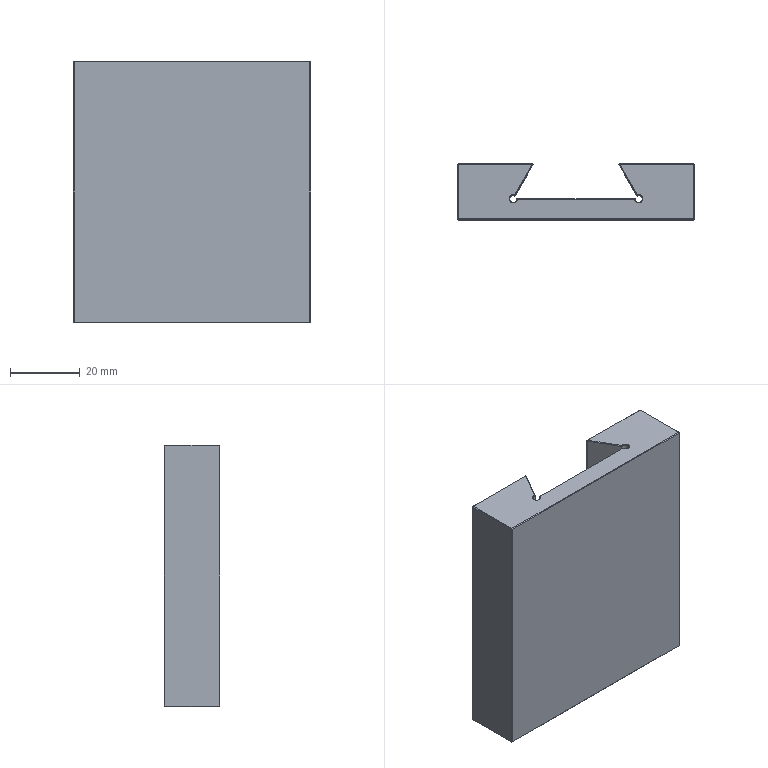Part | STEP file | 2006 | 1 solid | 43 faces | box 68 x 16 x 75 mm | volume 58521 mm3 | plane 32 | cone 8 | cylinder 3 | commonest cylinder face diameters 2 x3